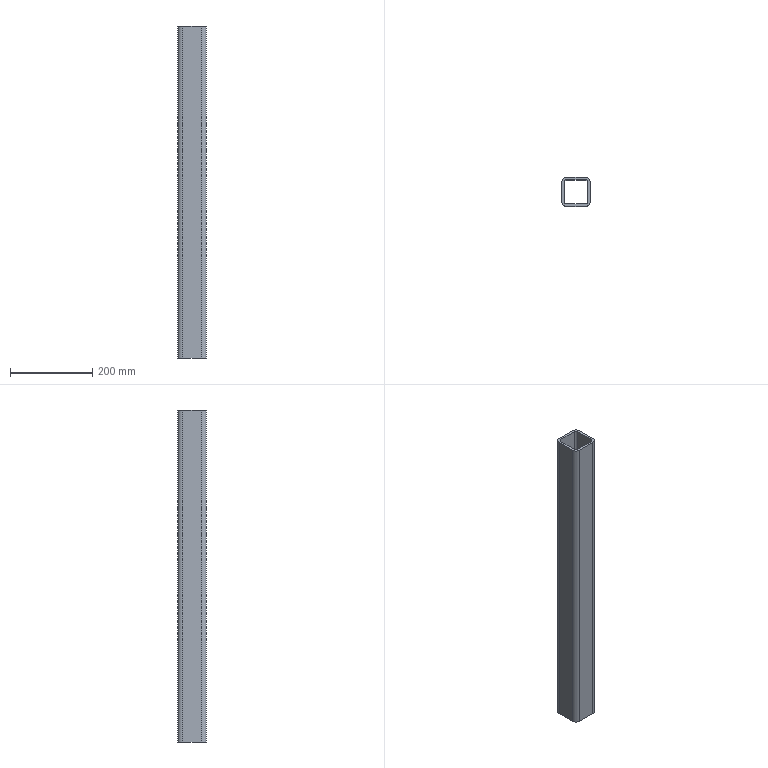Part | SolidWorks | features Extrusion 1 | 1 solid | 18 faces | box 70 x 70 x 805 mm | volume 1161850 mm3 | plane 10 | cylinder 8 | commonest cylinder face diameters 12 x4 24 x4
STEP:
#1=CARTESIAN_POINT('',(0.,12.,805.));
#2=VERTEX_POINT('',#1);
#3=CARTESIAN_POINT('',(12.,0.,805.));
#4=VERTEX_POINT('',#3);
#5=CARTESIAN_POINT('',(12.,12.,805.));
#6=DIRECTION('',(0.,0.,1.));
#7=DIRECTION('',(-1.,0.,0.));
#8=AXIS2_PLACEMENT_3D('',#5,#6,#7);
#9=CIRCLE('',#8,12.);
#10=EDGE_CURVE('',#2,#4,#9,.T.);
#11=ORIENTED_EDGE('',*,*,#10,.T.);
#12=CARTESIAN_POINT('',(58.,0.,805.));
#13=VERTEX_POINT('',#12);
#14=CARTESIAN_POINT('',(12.,0.,805.));
#15=DIRECTION('',(1.,0.,0.));
#16=VECTOR('',#15,1000.);
#17=LINE('',#14,#16);
#18=EDGE_CURVE('',#4,#13,#17,.T.);
#19=ORIENTED_EDGE('',*,*,#18,.T.);
#20=CARTESIAN_POINT('',(70.,12.,805.));
#21=VERTEX_POINT('',#20);
#22=CARTESIAN_POINT('',(58.,12.,805.));
#23=DIRECTION('',(0.,0.,1.));
#24=DIRECTION('',(1.,0.,0.));
#25=AXIS2_PLACEMENT_3D('',#22,#23,#24);
#26=CIRCLE('',#25,12.);
#27=EDGE_CURVE('',#13,#21,#26,.T.);
#28=ORIENTED_EDGE('',*,*,#27,.T.);
#29=CARTESIAN_POINT('',(70.,58.,805.));
#30=VERTEX_POINT('',#29);
#31=CARTESIAN_POINT('',(70.,12.,805.));
#32=DIRECTION('',(0.,1.,0.));
#33=VECTOR('',#32,1000.);
#34=LINE('',#31,#33);
#35=EDGE_CURVE('',#21,#30,#34,.T.);
#36=ORIENTED_EDGE('',*,*,#35,.T.);
#37=CARTESIAN_POINT('',(58.,70.,805.));
#38=VERTEX_POINT('',#37);
#39=CARTESIAN_POINT('',(58.,58.,805.));
#40=DIRECTION('',(0.,0.,1.));
#41=DIRECTION('',(-1.,0.,0.));
#42=AXIS2_PLACEMENT_3D('',#39,#40,#41);
#43=CIRCLE('',#42,12.);
#44=EDGE_CURVE('',#30,#38,#43,.T.);
#45=ORIENTED_EDGE('',*,*,#44,.T.);
#46=CARTESIAN_POINT('',(12.,70.,805.));
#47=VERTEX_POINT('',#46);
#48=CARTESIAN_POINT('',(12.,70.,805.));
#49=DIRECTION('',(-1.,0.,0.));
#50=VECTOR('',#49,1000.);
#51=LINE('',#48,#50);
#52=EDGE_CURVE('',#38,#47,#51,.T.);
#53=ORIENTED_EDGE('',*,*,#52,.T.);
#54=CARTESIAN_POINT('',(0.,58.,805.));
#55=VERTEX_POINT('',#54);
#56=CARTESIAN_POINT('',(12.,58.,805.));
#57=DIRECTION('',(0.,0.,1.));
#58=DIRECTION('',(-1.,0.,0.));
#59=AXIS2_PLACEMENT_3D('',#56,#57,#58);
#60=CIRCLE('',#59,12.);
#61=EDGE_CURVE('',#47,#55,#60,.T.);
#62=ORIENTED_EDGE('',*,*,#61,.T.);
#63=CARTESIAN_POINT('',(0.,12.,805.));
#64=DIRECTION('',(0.,-1.,0.));
#65=VECTOR('',#64,1000.);
#66=LINE('',#63,#65);
#67=EDGE_CURVE('',#55,#2,#66,.T.);
#68=ORIENTED_EDGE('',*,*,#67,.T.);
#69=EDGE_LOOP('',(#11,#19,#28,#36,#45,#53,#62,#68));
#70=FACE_OUTER_BOUND('',#69,.T.);
#71=CARTESIAN_POINT('',(6.,12.,805.));
#72=VERTEX_POINT('',#71);
#73=CARTESIAN_POINT('',(12.,6.,805.));
#74=VERTEX_POINT('',#73);
#75=CARTESIAN_POINT('',(12.,12.,805.));
#76=DIRECTION('',(0.,0.,1.));
#77=DIRECTION('',(-1.,0.,0.));
#78=AXIS2_PLACEMENT_3D('',#75,#76,#77);
#79=CIRCLE('',#78,6.);
#80=EDGE_CURVE('',#72,#74,#79,.T.);
#81=ORIENTED_EDGE('',*,*,#80,.F.);
#82=CARTESIAN_POINT('',(6.,58.,805.));
#83=VERTEX_POINT('',#82);
#84=CARTESIAN_POINT('',(6.,12.,805.));
#85=DIRECTION('',(0.,-1.,0.));
#86=VECTOR('',#85,1000.);
#87=LINE('',#84,#86);
#88=EDGE_CURVE('',#83,#72,#87,.T.);
#89=ORIENTED_EDGE('',*,*,#88,.F.);
#90=CARTESIAN_POINT('',(12.,64.,805.));
#91=VERTEX_POINT('',#90);
#92=CARTESIAN_POINT('',(12.,58.,805.));
#93=DIRECTION('',(0.,0.,1.));
#94=DIRECTION('',(-1.,0.,0.));
#95=AXIS2_PLACEMENT_3D('',#92,#93,#94);
#96=CIRCLE('',#95,6.);
#97=EDGE_CURVE('',#91,#83,#96,.T.);
#98=ORIENTED_EDGE('',*,*,#97,.F.);
#99=CARTESIAN_POINT('',(58.,64.,805.));
#100=VERTEX_POINT('',#99);
#101=CARTESIAN_POINT('',(12.,64.,805.));
#102=DIRECTION('',(-1.,0.,0.));
#103=VECTOR('',#102,1000.);
#104=LINE('',#101,#103);
#105=EDGE_CURVE('',#100,#91,#104,.T.);
#106=ORIENTED_EDGE('',*,*,#105,.F.);
#107=CARTESIAN_POINT('',(64.,58.,805.));
#108=VERTEX_POINT('',#107);
#109=CARTESIAN_POINT('',(58.,58.,805.));
#110=DIRECTION('',(0.,0.,1.));
#111=DIRECTION('',(-1.,0.,0.));
#112=AXIS2_PLACEMENT_3D('',#109,#110,#111);
#113=CIRCLE('',#112,6.);
#114=EDGE_CURVE('',#108,#100,#113,.T.);
#115=ORIENTED_EDGE('',*,*,#114,.F.);
#116=CARTESIAN_POINT('',(64.,12.,805.));
#117=VERTEX_POINT('',#116);
#118=CARTESIAN_POINT('',(64.,12.,805.));
#119=DIRECTION('',(0.,1.,0.));
#120=VECTOR('',#119,1000.);
#121=LINE('',#118,#120);
#122=EDGE_CURVE('',#117,#108,#121,.T.);
#123=ORIENTED_EDGE('',*,*,#122,.F.);
#124=CARTESIAN_POINT('',(58.,6.,805.));
#125=VERTEX_POINT('',#124);
#126=CARTESIAN_POINT('',(58.,12.,805.));
#127=DIRECTION('',(0.,0.,1.));
#128=DIRECTION('',(1.,0.,0.));
#129=AXIS2_PLACEMENT_3D('',#126,#127,#128);
#130=CIRCLE('',#129,6.);
#131=EDGE_CURVE('',#125,#117,#130,.T.);
#132=ORIENTED_EDGE('',*,*,#131,.F.);
#133=CARTESIAN_POINT('',(12.,6.,805.));
#134=DIRECTION('',(1.,0.,0.));
#135=VECTOR('',#134,1000.);
#136=LINE('',#133,#135);
#137=EDGE_CURVE('',#74,#125,#136,.T.);
#138=ORIENTED_EDGE('',*,*,#137,.F.);
#139=EDGE_LOOP('',(#81,#89,#98,#106,#115,#123,#132,#138));
#140=FACE_BOUND('',#139,.T.);
#141=CARTESIAN_POINT('',(12.,12.,805.));
#142=DIRECTION('',(0.,0.,-1.));
#143=DIRECTION('',(-1.,0.,0.));
#144=AXIS2_PLACEMENT_3D('',#141,#142,#143);
#145=PLANE('',#144);
#146=ADVANCED_FACE('',(#70,#140),#145,.F.);
#147=CARTESIAN_POINT('',(0.,12.,0.));
#148=VERTEX_POINT('',#147);
#149=CARTESIAN_POINT('',(12.,0.,0.));
#150=VERTEX_POINT('',#149);
#151=CARTESIAN_POINT('',(12.,12.,0.));
#152=DIRECTION('',(0.,0.,1.));
#153=DIRECTION('',(-1.,0.,0.));
#154=AXIS2_PLACEMENT_3D('',#151,#152,#153);
#155=CIRCLE('',#154,12.);
#156=EDGE_CURVE('',#148,#150,#155,.T.);
#157=ORIENTED_EDGE('',*,*,#156,.F.);
#158=CARTESIAN_POINT('',(0.,58.,0.));
#159=VERTEX_POINT('',#158);
#160=CARTESIAN_POINT('',(0.,12.,0.));
#161=DIRECTION('',(0.,-1.,0.));
#162=VECTOR('',#161,1000.);
#163=LINE('',#160,#162);
#164=EDGE_CURVE('',#159,#148,#163,.T.);
#165=ORIENTED_EDGE('',*,*,#164,.F.);
#166=CARTESIAN_POINT('',(12.,70.,0.));
#167=VERTEX_POINT('',#166);
#168=CARTESIAN_POINT('',(12.,58.,0.));
#169=DIRECTION('',(0.,0.,1.));
#170=DIRECTION('',(-1.,0.,0.));
#171=AXIS2_PLACEMENT_3D('',#168,#169,#170);
#172=CIRCLE('',#171,12.);
#173=EDGE_CURVE('',#167,#159,#172,.T.);
#174=ORIENTED_EDGE('',*,*,#173,.F.);
#175=CARTESIAN_POINT('',(58.,70.,0.));
#176=VERTEX_POINT('',#175);
#177=CARTESIAN_POINT('',(12.,70.,0.));
#178=DIRECTION('',(-1.,0.,0.));
#179=VECTOR('',#178,1000.);
#180=LINE('',#177,#179);
#181=EDGE_CURVE('',#176,#167,#180,.T.);
#182=ORIENTED_EDGE('',*,*,#181,.F.);
#183=CARTESIAN_POINT('',(70.,58.,0.));
#184=VERTEX_POINT('',#183);
#185=CARTESIAN_POINT('',(58.,58.,0.));
#186=DIRECTION('',(0.,0.,1.));
#187=DIRECTION('',(-1.,0.,0.));
#188=AXIS2_PLACEMENT_3D('',#185,#186,#187);
#189=CIRCLE('',#188,12.);
#190=EDGE_CURVE('',#184,#176,#189,.T.);
#191=ORIENTED_EDGE('',*,*,#190,.F.);
#192=CARTESIAN_POINT('',(70.,12.,0.));
#193=VERTEX_POINT('',#192);
#194=CARTESIAN_POINT('',(70.,12.,0.));
#195=DIRECTION('',(0.,1.,0.));
#196=VECTOR('',#195,1000.);
#197=LINE('',#194,#196);
#198=EDGE_CURVE('',#193,#184,#197,.T.);
#199=ORIENTED_EDGE('',*,*,#198,.F.);
#200=CARTESIAN_POINT('',(58.,0.,0.));
#201=VERTEX_POINT('',#200);
#202=CARTESIAN_POINT('',(58.,12.,0.));
#203=DIRECTION('',(0.,0.,1.));
#204=DIRECTION('',(1.,0.,0.));
#205=AXIS2_PLACEMENT_3D('',#202,#203,#204);
#206=CIRCLE('',#205,12.);
#207=EDGE_CURVE('',#201,#193,#206,.T.);
#208=ORIENTED_EDGE('',*,*,#207,.F.);
#209=CARTESIAN_POINT('',(12.,0.,0.));
#210=DIRECTION('',(1.,0.,0.));
#211=VECTOR('',#210,1000.);
#212=LINE('',#209,#211);
#213=EDGE_CURVE('',#150,#201,#212,.T.);
#214=ORIENTED_EDGE('',*,*,#213,.F.);
#215=EDGE_LOOP('',(#157,#165,#174,#182,#191,#199,#208,#214));
#216=FACE_OUTER_BOUND('',#215,.T.);
#217=CARTESIAN_POINT('',(6.,58.,0.));
#218=VERTEX_POINT('',#217);
#219=CARTESIAN_POINT('',(6.,12.,0.));
#220=VERTEX_POINT('',#219);
#221=CARTESIAN_POINT('',(6.,12.,0.));
#222=DIRECTION('',(0.,-1.,0.));
#223=VECTOR('',#222,1000.);
#224=LINE('',#221,#223);
#225=EDGE_CURVE('',#218,#220,#224,.T.);
#226=ORIENTED_EDGE('',*,*,#225,.T.);
#227=CARTESIAN_POINT('',(12.,6.,0.));
#228=VERTEX_POINT('',#227);
#229=CARTESIAN_POINT('',(12.,12.,0.));
#230=DIRECTION('',(0.,0.,1.));
#231=DIRECTION('',(-1.,0.,0.));
#232=AXIS2_PLACEMENT_3D('',#229,#230,#231);
#233=CIRCLE('',#232,6.);
#234=EDGE_CURVE('',#220,#228,#233,.T.);
#235=ORIENTED_EDGE('',*,*,#234,.T.);
#236=CARTESIAN_POINT('',(58.,6.,0.));
#237=VERTEX_POINT('',#236);
#238=CARTESIAN_POINT('',(12.,6.,0.));
#239=DIRECTION('',(1.,0.,0.));
#240=VECTOR('',#239,1000.);
#241=LINE('',#238,#240);
#242=EDGE_CURVE('',#228,#237,#241,.T.);
#243=ORIENTED_EDGE('',*,*,#242,.T.);
#244=CARTESIAN_POINT('',(64.,12.,0.));
#245=VERTEX_POINT('',#244);
#246=CARTESIAN_POINT('',(58.,12.,0.));
#247=DIRECTION('',(0.,0.,1.));
#248=DIRECTION('',(1.,0.,0.));
#249=AXIS2_PLACEMENT_3D('',#246,#247,#248);
#250=CIRCLE('',#249,6.);
#251=EDGE_CURVE('',#237,#245,#250,.T.);
#252=ORIENTED_EDGE('',*,*,#251,.T.);
#253=CARTESIAN_POINT('',(64.,58.,0.));
#254=VERTEX_POINT('',#253);
#255=CARTESIAN_POINT('',(64.,12.,0.));
#256=DIRECTION('',(0.,1.,0.));
#257=VECTOR('',#256,1000.);
#258=LINE('',#255,#257);
#259=EDGE_CURVE('',#245,#254,#258,.T.);
#260=ORIENTED_EDGE('',*,*,#259,.T.);
#261=CARTESIAN_POINT('',(58.,64.,0.));
#262=VERTEX_POINT('',#261);
#263=CARTESIAN_POINT('',(58.,58.,0.));
#264=DIRECTION('',(0.,0.,1.));
#265=DIRECTION('',(-1.,0.,0.));
#266=AXIS2_PLACEMENT_3D('',#263,#264,#265);
#267=CIRCLE('',#266,6.);
#268=EDGE_CURVE('',#254,#262,#267,.T.);
#269=ORIENTED_EDGE('',*,*,#268,.T.);
#270=CARTESIAN_POINT('',(12.,64.,0.));
#271=VERTEX_POINT('',#270);
#272=CARTESIAN_POINT('',(12.,64.,0.));
#273=DIRECTION('',(-1.,0.,0.));
#274=VECTOR('',#273,1000.);
#275=LINE('',#272,#274);
#276=EDGE_CURVE('',#262,#271,#275,.T.);
#277=ORIENTED_EDGE('',*,*,#276,.T.);
#278=CARTESIAN_POINT('',(12.,58.,0.));
#279=DIRECTION('',(0.,0.,1.));
#280=DIRECTION('',(-1.,0.,0.));
#281=AXIS2_PLACEMENT_3D('',#278,#279,#280);
#282=CIRCLE('',#281,6.);
#283=EDGE_CURVE('',#271,#218,#282,.T.);
#284=ORIENTED_EDGE('',*,*,#283,.T.);
#285=EDGE_LOOP('',(#226,#235,#243,#252,#260,#269,#277,#284));
#286=FACE_BOUND('',#285,.T.);
#287=CARTESIAN_POINT('',(12.,12.,0.));
#288=DIRECTION('',(0.,0.,-1.));
#289=DIRECTION('',(-1.,0.,0.));
#290=AXIS2_PLACEMENT_3D('',#287,#288,#289);
#291=PLANE('',#290);
#292=ADVANCED_FACE('',(#216,#286),#291,.T.);
#293=ORIENTED_EDGE('',*,*,#156,.T.);
#294=CARTESIAN_POINT('',(12.,0.,805.));
#295=DIRECTION('',(0.,0.,-1.));
#296=VECTOR('',#295,1000.);
#297=LINE('',#294,#296);
#298=EDGE_CURVE('',#4,#150,#297,.T.);
#299=ORIENTED_EDGE('',*,*,#298,.F.);
#300=ORIENTED_EDGE('',*,*,#10,.F.);
#301=CARTESIAN_POINT('',(0.,12.,805.));
#302=DIRECTION('',(0.,0.,-1.));
#303=VECTOR('',#302,1000.);
#304=LINE('',#301,#303);
#305=EDGE_CURVE('',#2,#148,#304,.T.);
#306=ORIENTED_EDGE('',*,*,#305,.T.);
#307=EDGE_LOOP('',(#293,#299,#300,#306));
#308=FACE_OUTER_BOUND('',#307,.T.);
#309=CARTESIAN_POINT('',(12.,12.,805.));
#310=DIRECTION('',(0.,0.,-1.));
#311=DIRECTION('',(-1.,0.,0.));
#312=AXIS2_PLACEMENT_3D('',#309,#310,#311);
#313=CYLINDRICAL_SURFACE('',#312,12.);
#314=ADVANCED_FACE('',(#308),#313,.T.);
#315=ORIENTED_EDGE('',*,*,#213,.T.);
#316=CARTESIAN_POINT('',(58.,0.,805.));
#317=DIRECTION('',(0.,0.,-1.));
#318=VECTOR('',#317,1000.);
#319=LINE('',#316,#318);
#320=EDGE_CURVE('',#13,#201,#319,.T.);
#321=ORIENTED_EDGE('',*,*,#320,.F.);
#322=ORIENTED_EDGE('',*,*,#18,.F.);
#323=ORIENTED_EDGE('',*,*,#298,.T.);
#324=EDGE_LOOP('',(#315,#321,#322,#323));
#325=FACE_OUTER_BOUND('',#324,.T.);
#326=CARTESIAN_POINT('',(12.,0.,805.));
#327=DIRECTION('',(0.,1.,0.));
#328=DIRECTION('',(0.,0.,1.));
#329=AXIS2_PLACEMENT_3D('',#326,#327,#328);
#330=PLANE('',#329);
#331=ADVANCED_FACE('',(#325),#330,.F.);
#332=ORIENTED_EDGE('',*,*,#207,.T.);
#333=CARTESIAN_POINT('',(70.,12.,805.));
#334=DIRECTION('',(0.,0.,-1.));
#335=VECTOR('',#334,1000.);
#336=LINE('',#333,#335);
#337=EDGE_CURVE('',#21,#193,#336,.T.);
#338=ORIENTED_EDGE('',*,*,#337,.F.);
#339=ORIENTED_EDGE('',*,*,#27,.F.);
#340=ORIENTED_EDGE('',*,*,#320,.T.);
#341=EDGE_LOOP('',(#332,#338,#339,#340));
#342=FACE_OUTER_BOUND('',#341,.T.);
#343=CARTESIAN_POINT('',(58.,12.,805.));
#344=DIRECTION('',(0.,0.,-1.));
#345=DIRECTION('',(-1.,0.,0.));
#346=AXIS2_PLACEMENT_3D('',#343,#344,#345);
#347=CYLINDRICAL_SURFACE('',#346,12.);
#348=ADVANCED_FACE('',(#342),#347,.T.);
#349=ORIENTED_EDGE('',*,*,#198,.T.);
#350=CARTESIAN_POINT('',(70.,58.,805.));
#351=DIRECTION('',(0.,0.,-1.));
#352=VECTOR('',#351,1000.);
#353=LINE('',#350,#352);
#354=EDGE_CURVE('',#30,#184,#353,.T.);
#355=ORIENTED_EDGE('',*,*,#354,.F.);
#356=ORIENTED_EDGE('',*,*,#35,.F.);
#357=ORIENTED_EDGE('',*,*,#337,.T.);
#358=EDGE_LOOP('',(#349,#355,#356,#357));
#359=FACE_OUTER_BOUND('',#358,.T.);
#360=CARTESIAN_POINT('',(70.,12.,805.));
#361=DIRECTION('',(-1.,0.,0.));
#362=DIRECTION('',(0.,0.,1.));
#363=AXIS2_PLACEMENT_3D('',#360,#361,#362);
#364=PLANE('',#363);
#365=ADVANCED_FACE('',(#359),#364,.F.);
#366=ORIENTED_EDGE('',*,*,#190,.T.);
#367=CARTESIAN_POINT('',(58.,70.,805.));
#368=DIRECTION('',(0.,0.,-1.));
#369=VECTOR('',#368,1000.);
#370=LINE('',#367,#369);
#371=EDGE_CURVE('',#38,#176,#370,.T.);
#372=ORIENTED_EDGE('',*,*,#371,.F.);
#373=ORIENTED_EDGE('',*,*,#44,.F.);
#374=ORIENTED_EDGE('',*,*,#354,.T.);
#375=EDGE_LOOP('',(#366,#372,#373,#374));
#376=FACE_OUTER_BOUND('',#375,.T.);
#377=CARTESIAN_POINT('',(58.,58.,805.));
#378=DIRECTION('',(0.,0.,-1.));
#379=DIRECTION('',(-1.,0.,0.));
#380=AXIS2_PLACEMENT_3D('',#377,#378,#379);
#381=CYLINDRICAL_SURFACE('',#380,12.);
#382=ADVANCED_FACE('',(#376),#381,.T.);
#383=ORIENTED_EDGE('',*,*,#181,.T.);
#384=CARTESIAN_POINT('',(12.,70.,805.));
#385=DIRECTION('',(0.,0.,-1.));
#386=VECTOR('',#385,1000.);
#387=LINE('',#384,#386);
#388=EDGE_CURVE('',#47,#167,#387,.T.);
#389=ORIENTED_EDGE('',*,*,#388,.F.);
#390=ORIENTED_EDGE('',*,*,#52,.F.);
#391=ORIENTED_EDGE('',*,*,#371,.T.);
#392=EDGE_LOOP('',(#383,#389,#390,#391));
#393=FACE_OUTER_BOUND('',#392,.T.);
#394=CARTESIAN_POINT('',(12.,70.,805.));
#395=DIRECTION('',(0.,-1.,0.));
#396=DIRECTION('',(0.,0.,-1.));
#397=AXIS2_PLACEMENT_3D('',#394,#395,#396);
#398=PLANE('',#397);
#399=ADVANCED_FACE('',(#393),#398,.F.);
#400=ORIENTED_EDGE('',*,*,#173,.T.);
#401=CARTESIAN_POINT('',(0.,58.,805.));
#402=DIRECTION('',(0.,0.,-1.));
#403=VECTOR('',#402,1000.);
#404=LINE('',#401,#403);
#405=EDGE_CURVE('',#55,#159,#404,.T.);
#406=ORIENTED_EDGE('',*,*,#405,.F.);
#407=ORIENTED_EDGE('',*,*,#61,.F.);
#408=ORIENTED_EDGE('',*,*,#388,.T.);
#409=EDGE_LOOP('',(#400,#406,#407,#408));
#410=FACE_OUTER_BOUND('',#409,.T.);
#411=CARTESIAN_POINT('',(12.,58.,805.));
#412=DIRECTION('',(0.,0.,-1.));
#413=DIRECTION('',(-1.,0.,0.));
#414=AXIS2_PLACEMENT_3D('',#411,#412,#413);
#415=CYLINDRICAL_SURFACE('',#414,12.);
#416=ADVANCED_FACE('',(#410),#415,.T.);
#417=ORIENTED_EDGE('',*,*,#164,.T.);
#418=ORIENTED_EDGE('',*,*,#305,.F.);
#419=ORIENTED_EDGE('',*,*,#67,.F.);
#420=ORIENTED_EDGE('',*,*,#405,.T.);
#421=EDGE_LOOP('',(#417,#418,#419,#420));
#422=FACE_OUTER_BOUND('',#421,.T.);
#423=CARTESIAN_POINT('',(0.,12.,805.));
#424=DIRECTION('',(1.,0.,0.));
#425=DIRECTION('',(0.,0.,-1.));
#426=AXIS2_PLACEMENT_3D('',#423,#424,#425);
#427=PLANE('',#426);
#428=ADVANCED_FACE('',(#422),#427,.F.);
#429=ORIENTED_EDGE('',*,*,#234,.F.);
#430=CARTESIAN_POINT('',(6.,12.,805.));
#431=DIRECTION('',(0.,0.,-1.));
#432=VECTOR('',#431,1000.);
#433=LINE('',#430,#432);
#434=EDGE_CURVE('',#72,#220,#433,.T.);
#435=ORIENTED_EDGE('',*,*,#434,.F.);
#436=ORIENTED_EDGE('',*,*,#80,.T.);
#437=CARTESIAN_POINT('',(12.,6.,805.));
#438=DIRECTION('',(0.,0.,-1.));
#439=VECTOR('',#438,1000.);
#440=LINE('',#437,#439);
#441=EDGE_CURVE('',#74,#228,#440,.T.);
#442=ORIENTED_EDGE('',*,*,#441,.T.);
#443=EDGE_LOOP('',(#429,#435,#436,#442));
#444=FACE_OUTER_BOUND('',#443,.T.);
#445=CARTESIAN_POINT('',(12.,12.,805.));
#446=DIRECTION('',(0.,0.,-1.));
#447=DIRECTION('',(-1.,0.,0.));
#448=AXIS2_PLACEMENT_3D('',#445,#446,#447);
#449=CYLINDRICAL_SURFACE('',#448,6.);
#450=ADVANCED_FACE('',(#444),#449,.F.);
#451=ORIENTED_EDGE('',*,*,#242,.F.);
#452=ORIENTED_EDGE('',*,*,#441,.F.);
#453=ORIENTED_EDGE('',*,*,#137,.T.);
#454=CARTESIAN_POINT('',(58.,6.,805.));
#455=DIRECTION('',(0.,0.,-1.));
#456=VECTOR('',#455,1000.);
#457=LINE('',#454,#456);
#458=EDGE_CURVE('',#125,#237,#457,.T.);
#459=ORIENTED_EDGE('',*,*,#458,.T.);
#460=EDGE_LOOP('',(#451,#452,#453,#459));
#461=FACE_OUTER_BOUND('',#460,.T.);
#462=CARTESIAN_POINT('',(12.,6.,805.));
#463=DIRECTION('',(0.,1.,0.));
#464=DIRECTION('',(0.,0.,1.));
#465=AXIS2_PLACEMENT_3D('',#462,#463,#464);
#466=PLANE('',#465);
#467=ADVANCED_FACE('',(#461),#466,.T.);
#468=ORIENTED_EDGE('',*,*,#251,.F.);
#469=ORIENTED_EDGE('',*,*,#458,.F.);
#470=ORIENTED_EDGE('',*,*,#131,.T.);
#471=CARTESIAN_POINT('',(64.,12.,805.));
#472=DIRECTION('',(0.,0.,-1.));
#473=VECTOR('',#472,1000.);
#474=LINE('',#471,#473);
#475=EDGE_CURVE('',#117,#245,#474,.T.);
#476=ORIENTED_EDGE('',*,*,#475,.T.);
#477=EDGE_LOOP('',(#468,#469,#470,#476));
#478=FACE_OUTER_BOUND('',#477,.T.);
#479=CARTESIAN_POINT('',(58.,12.,805.));
#480=DIRECTION('',(0.,0.,-1.));
#481=DIRECTION('',(-1.,0.,0.));
#482=AXIS2_PLACEMENT_3D('',#479,#480,#481);
#483=CYLINDRICAL_SURFACE('',#482,6.);
#484=ADVANCED_FACE('',(#478),#483,.F.);
#485=ORIENTED_EDGE('',*,*,#259,.F.);
#486=ORIENTED_EDGE('',*,*,#475,.F.);
#487=ORIENTED_EDGE('',*,*,#122,.T.);
#488=CARTESIAN_POINT('',(64.,58.,805.));
#489=DIRECTION('',(0.,0.,-1.));
#490=VECTOR('',#489,1000.);
#491=LINE('',#488,#490);
#492=EDGE_CURVE('',#108,#254,#491,.T.);
#493=ORIENTED_EDGE('',*,*,#492,.T.);
#494=EDGE_LOOP('',(#485,#486,#487,#493));
#495=FACE_OUTER_BOUND('',#494,.T.);
#496=CARTESIAN_POINT('',(64.,12.,805.));
#497=DIRECTION('',(-1.,0.,0.));
#498=DIRECTION('',(0.,0.,1.));
#499=AXIS2_PLACEMENT_3D('',#496,#497,#498);
#500=PLANE('',#499);
#501=ADVANCED_FACE('',(#495),#500,.T.);
#502=ORIENTED_EDGE('',*,*,#268,.F.);
#503=ORIENTED_EDGE('',*,*,#492,.F.);
#504=ORIENTED_EDGE('',*,*,#114,.T.);
#505=CARTESIAN_POINT('',(58.,64.,805.));
#506=DIRECTION('',(0.,0.,-1.));
#507=VECTOR('',#506,1000.);
#508=LINE('',#505,#507);
#509=EDGE_CURVE('',#100,#262,#508,.T.);
#510=ORIENTED_EDGE('',*,*,#509,.T.);
#511=EDGE_LOOP('',(#502,#503,#504,#510));
#512=FACE_OUTER_BOUND('',#511,.T.);
#513=CARTESIAN_POINT('',(58.,58.,805.));
#514=DIRECTION('',(0.,0.,-1.));
#515=DIRECTION('',(-1.,0.,0.));
#516=AXIS2_PLACEMENT_3D('',#513,#514,#515);
#517=CYLINDRICAL_SURFACE('',#516,6.);
#518=ADVANCED_FACE('',(#512),#517,.F.);
#519=ORIENTED_EDGE('',*,*,#276,.F.);
#520=ORIENTED_EDGE('',*,*,#509,.F.);
#521=ORIENTED_EDGE('',*,*,#105,.T.);
#522=CARTESIAN_POINT('',(12.,64.,805.));
#523=DIRECTION('',(0.,0.,-1.));
#524=VECTOR('',#523,1000.);
#525=LINE('',#522,#524);
#526=EDGE_CURVE('',#91,#271,#525,.T.);
#527=ORIENTED_EDGE('',*,*,#526,.T.);
#528=EDGE_LOOP('',(#519,#520,#521,#527));
#529=FACE_OUTER_BOUND('',#528,.T.);
#530=CARTESIAN_POINT('',(12.,64.,805.));
#531=DIRECTION('',(0.,-1.,0.));
#532=DIRECTION('',(0.,0.,-1.));
#533=AXIS2_PLACEMENT_3D('',#530,#531,#532);
#534=PLANE('',#533);
#535=ADVANCED_FACE('',(#529),#534,.T.);
#536=ORIENTED_EDGE('',*,*,#283,.F.);
#537=ORIENTED_EDGE('',*,*,#526,.F.);
#538=ORIENTED_EDGE('',*,*,#97,.T.);
#539=CARTESIAN_POINT('',(6.,58.,805.));
#540=DIRECTION('',(0.,0.,-1.));
#541=VECTOR('',#540,1000.);
#542=LINE('',#539,#541);
#543=EDGE_CURVE('',#83,#218,#542,.T.);
#544=ORIENTED_EDGE('',*,*,#543,.T.);
#545=EDGE_LOOP('',(#536,#537,#538,#544));
#546=FACE_OUTER_BOUND('',#545,.T.);
#547=CARTESIAN_POINT('',(12.,58.,805.));
#548=DIRECTION('',(0.,0.,-1.));
#549=DIRECTION('',(-1.,0.,0.));
#550=AXIS2_PLACEMENT_3D('',#547,#548,#549);
#551=CYLINDRICAL_SURFACE('',#550,6.);
#552=ADVANCED_FACE('',(#546),#551,.F.);
#553=ORIENTED_EDGE('',*,*,#225,.F.);
#554=ORIENTED_EDGE('',*,*,#543,.F.);
#555=ORIENTED_EDGE('',*,*,#88,.T.);
#556=ORIENTED_EDGE('',*,*,#434,.T.);
#557=EDGE_LOOP('',(#553,#554,#555,#556));
#558=FACE_OUTER_BOUND('',#557,.T.);
#559=CARTESIAN_POINT('',(6.,12.,805.));
#560=DIRECTION('',(1.,0.,0.));
#561=DIRECTION('',(0.,0.,-1.));
#562=AXIS2_PLACEMENT_3D('',#559,#560,#561);
#563=PLANE('',#562);
#564=ADVANCED_FACE('',(#558),#563,.T.);
#565=CLOSED_SHELL('',(#146,#292,#314,#331,#348,#365,#382,#399,#416,#428,#450,#467,#484,#501,#518,#535,#552,#564));
#566=MANIFOLD_SOLID_BREP('',#565);
#567=CARTESIAN_POINT('',(0.,0.,0.));
#568=DIRECTION('',(0.,0.,1.));
#569=DIRECTION('',(1.,0.,0.));
#570=AXIS2_PLACEMENT_3D('',#567,#568,#569);
#571=(LENGTH_UNIT()NAMED_UNIT(*)SI_UNIT(.MILLI.,.METRE.));
#572=UNCERTAINTY_MEASURE_WITH_UNIT(LENGTH_MEASURE(0.00001),#571,'','');
#573=(NAMED_UNIT(*)PLANE_ANGLE_UNIT()SI_UNIT($,.RADIAN.));
#574=(NAMED_UNIT(*)SI_UNIT($,.STERADIAN.)SOLID_ANGLE_UNIT());
#575=(GEOMETRIC_REPRESENTATION_CONTEXT(3)GLOBAL_UNCERTAINTY_ASSIGNED_CONTEXT((#572))GLOBAL_UNIT_ASSIGNED_CONTEXT((#571,#573,#574))REPRESENTATION_CONTEXT('',''));
#576=ADVANCED_BREP_SHAPE_REPRESENTATION('',(#566,#570),#575);